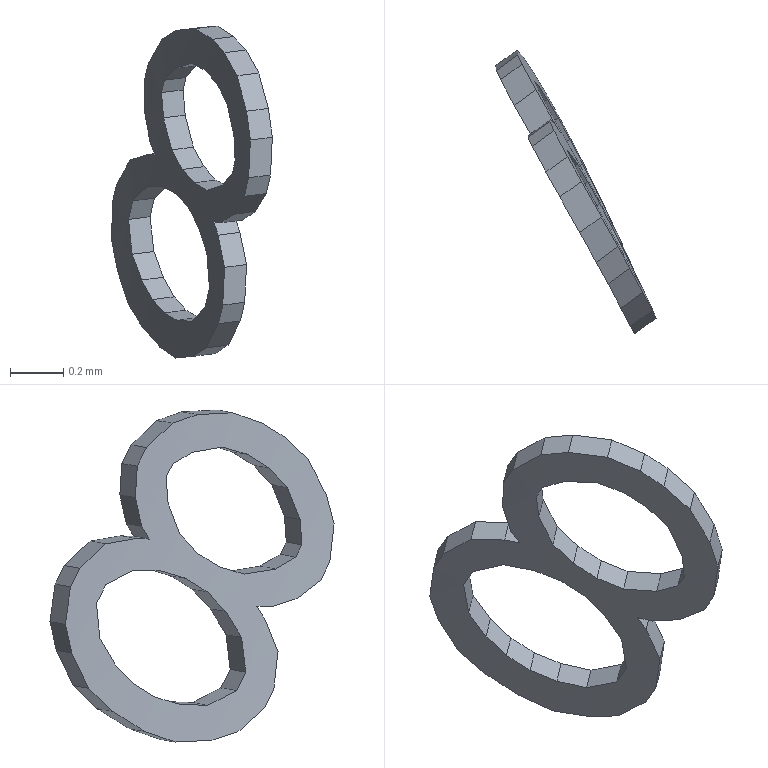Part | SolidWorks | features BaseBody 1 | 1 solid | 68 faces | box 0.6045 x 1.069 x 1.25 mm | volume 0.05056 mm3 | plane 66 | cylinder 2 | commonest cylinder face diameters 16.8 x1 17 x1